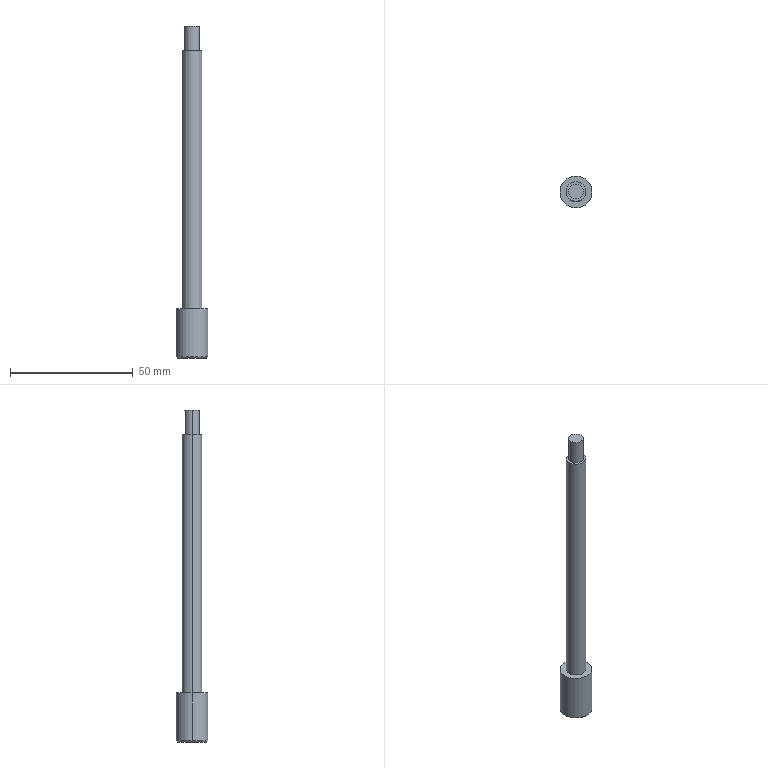Part | SolidWorks | features ICE 2, Chamfer 1, Extrusion 1, HoleWzd 1 | 1 solid | 20 faces | box 13 x 13 x 135 mm | volume 8178 mm3 | cylinder 10 | cone 6 | plane 4 | commonest cylinder face diameters 2 x4 6 x2 8 x2 13 x2
STEP:
#1=CARTESIAN_POINT('',(3.,0.,135.));
#2=VERTEX_POINT('',#1);
#3=CARTESIAN_POINT('',(-3.,0.,135.));
#4=VERTEX_POINT('',#3);
#5=CARTESIAN_POINT('',(0.,0.,135.));
#6=DIRECTION('',(0.,0.,1.));
#7=DIRECTION('',(1.,0.,0.));
#8=AXIS2_PLACEMENT_3D('',#5,#6,#7);
#9=CIRCLE('',#8,3.);
#10=EDGE_CURVE('',#2,#4,#9,.T.);
#11=ORIENTED_EDGE('',*,*,#10,.F.);
#12=CARTESIAN_POINT('',(3.,0.,125.));
#13=VERTEX_POINT('',#12);
#14=CARTESIAN_POINT('',(3.,0.,135.));
#15=DIRECTION('',(0.,0.,-1.));
#16=VECTOR('',#15,1000.);
#17=LINE('',#14,#16);
#18=EDGE_CURVE('',#2,#13,#17,.T.);
#19=ORIENTED_EDGE('',*,*,#18,.T.);
#20=CARTESIAN_POINT('',(-3.,0.,125.));
#21=VERTEX_POINT('',#20);
#22=CARTESIAN_POINT('',(0.,0.,125.));
#23=DIRECTION('',(0.,0.,1.));
#24=DIRECTION('',(1.,0.,0.));
#25=AXIS2_PLACEMENT_3D('',#22,#23,#24);
#26=CIRCLE('',#25,3.);
#27=EDGE_CURVE('',#13,#21,#26,.T.);
#28=ORIENTED_EDGE('',*,*,#27,.T.);
#29=CARTESIAN_POINT('',(-3.,0.,135.));
#30=DIRECTION('',(0.,0.,-1.));
#31=VECTOR('',#30,1000.);
#32=LINE('',#29,#31);
#33=EDGE_CURVE('',#4,#21,#32,.T.);
#34=ORIENTED_EDGE('',*,*,#33,.F.);
#35=EDGE_LOOP('',(#11,#19,#28,#34));
#36=FACE_OUTER_BOUND('',#35,.T.);
#37=CARTESIAN_POINT('',(0.,0.,135.));
#38=DIRECTION('',(0.,0.,-1.));
#39=DIRECTION('',(-1.,0.,0.));
#40=AXIS2_PLACEMENT_3D('',#37,#38,#39);
#41=CYLINDRICAL_SURFACE('',#40,3.);
#42=ADVANCED_FACE('',(#36),#41,.T.);
#43=CARTESIAN_POINT('',(4.,0.,125.));
#44=VERTEX_POINT('',#43);
#45=CARTESIAN_POINT('',(-4.,0.,125.));
#46=VERTEX_POINT('',#45);
#47=CARTESIAN_POINT('',(0.,0.,125.));
#48=DIRECTION('',(0.,0.,1.));
#49=DIRECTION('',(1.,0.,0.));
#50=AXIS2_PLACEMENT_3D('',#47,#48,#49);
#51=CIRCLE('',#50,4.);
#52=EDGE_CURVE('',#44,#46,#51,.T.);
#53=ORIENTED_EDGE('',*,*,#52,.F.);
#54=CARTESIAN_POINT('',(4.,0.,20.));
#55=VERTEX_POINT('',#54);
#56=CARTESIAN_POINT('',(4.,0.,125.));
#57=DIRECTION('',(0.,0.,-1.));
#58=VECTOR('',#57,1000.);
#59=LINE('',#56,#58);
#60=EDGE_CURVE('',#44,#55,#59,.T.);
#61=ORIENTED_EDGE('',*,*,#60,.T.);
#62=CARTESIAN_POINT('',(-4.,0.,20.));
#63=VERTEX_POINT('',#62);
#64=CARTESIAN_POINT('',(0.,0.,20.));
#65=DIRECTION('',(0.,0.,1.));
#66=DIRECTION('',(1.,0.,0.));
#67=AXIS2_PLACEMENT_3D('',#64,#65,#66);
#68=CIRCLE('',#67,4.);
#69=EDGE_CURVE('',#55,#63,#68,.T.);
#70=ORIENTED_EDGE('',*,*,#69,.T.);
#71=CARTESIAN_POINT('',(-4.,0.,125.));
#72=DIRECTION('',(0.,0.,-1.));
#73=VECTOR('',#72,1000.);
#74=LINE('',#71,#73);
#75=EDGE_CURVE('',#46,#63,#74,.T.);
#76=ORIENTED_EDGE('',*,*,#75,.F.);
#77=EDGE_LOOP('',(#53,#61,#70,#76));
#78=FACE_OUTER_BOUND('',#77,.T.);
#79=CARTESIAN_POINT('',(0.,0.,125.));
#80=DIRECTION('',(0.,0.,-1.));
#81=DIRECTION('',(-1.,0.,0.));
#82=AXIS2_PLACEMENT_3D('',#79,#80,#81);
#83=CYLINDRICAL_SURFACE('',#82,4.);
#84=ADVANCED_FACE('',(#78),#83,.T.);
#85=CARTESIAN_POINT('',(4.5,0.,5.));
#86=VERTEX_POINT('',#85);
#87=CARTESIAN_POINT('',(2.5,0.,5.));
#88=VERTEX_POINT('',#87);
#89=CARTESIAN_POINT('',(3.5,0.,5.));
#90=DIRECTION('',(0.,0.,-1.));
#91=DIRECTION('',(-1.,0.,0.));
#92=AXIS2_PLACEMENT_3D('',#89,#90,#91);
#93=CIRCLE('',#92,1.);
#94=EDGE_CURVE('',#86,#88,#93,.T.);
#95=ORIENTED_EDGE('',*,*,#94,.F.);
#96=CARTESIAN_POINT('',(4.5,0.,0.));
#97=VERTEX_POINT('',#96);
#98=CARTESIAN_POINT('',(4.5,0.,0.));
#99=DIRECTION('',(0.,0.,-1.));
#100=VECTOR('',#99,1000.);
#101=LINE('',#98,#100);
#102=EDGE_CURVE('',#86,#97,#101,.T.);
#103=ORIENTED_EDGE('',*,*,#102,.T.);
#104=CARTESIAN_POINT('',(2.5,0.,0.));
#105=VERTEX_POINT('',#104);
#106=CARTESIAN_POINT('',(3.5,0.,0.));
#107=DIRECTION('',(0.,0.,-1.));
#108=DIRECTION('',(-1.,0.,0.));
#109=AXIS2_PLACEMENT_3D('',#106,#107,#108);
#110=CIRCLE('',#109,1.);
#111=EDGE_CURVE('',#97,#105,#110,.T.);
#112=ORIENTED_EDGE('',*,*,#111,.T.);
#113=CARTESIAN_POINT('',(2.5,0.,0.));
#114=DIRECTION('',(0.,0.,-1.));
#115=VECTOR('',#114,1000.);
#116=LINE('',#113,#115);
#117=EDGE_CURVE('',#88,#105,#116,.T.);
#118=ORIENTED_EDGE('',*,*,#117,.F.);
#119=EDGE_LOOP('',(#95,#103,#112,#118));
#120=FACE_OUTER_BOUND('',#119,.T.);
#121=CARTESIAN_POINT('',(3.5,0.,0.));
#122=DIRECTION('',(0.,0.,-1.));
#123=DIRECTION('',(-1.,0.,0.));
#124=AXIS2_PLACEMENT_3D('',#121,#122,#123);
#125=CYLINDRICAL_SURFACE('',#124,1.);
#126=ADVANCED_FACE('',(#120),#125,.F.);
#127=CARTESIAN_POINT('',(3.5,0.,5.601));
#128=VERTEX_POINT('',#127);
#129=CARTESIAN_POINT('',(2.5,0.,5.));
#130=DIRECTION('',(-0.8572,0.,-0.515));
#131=VECTOR('',#130,1000.);
#132=LINE('',#129,#131);
#133=EDGE_CURVE('',#128,#88,#132,.T.);
#134=ORIENTED_EDGE('',*,*,#133,.F.);
#135=CARTESIAN_POINT('',(4.5,0.,5.));
#136=DIRECTION('',(0.8572,0.,-0.515));
#137=VECTOR('',#136,1000.);
#138=LINE('',#135,#137);
#139=EDGE_CURVE('',#128,#86,#138,.T.);
#140=ORIENTED_EDGE('',*,*,#139,.T.);
#141=ORIENTED_EDGE('',*,*,#94,.T.);
#142=EDGE_LOOP('',(#134,#140,#141));
#143=FACE_OUTER_BOUND('',#142,.T.);
#144=CARTESIAN_POINT('',(3.5,0.,5.));
#145=DIRECTION('',(0.,0.,-1.));
#146=DIRECTION('',(-1.,0.,0.));
#147=AXIS2_PLACEMENT_3D('',#144,#145,#146);
#148=CONICAL_SURFACE('',#147,1.,1.03);
#149=ADVANCED_FACE('',(#143),#148,.F.);
#150=CARTESIAN_POINT('',(-2.5,0.,5.));
#151=VERTEX_POINT('',#150);
#152=CARTESIAN_POINT('',(-4.5,0.,5.));
#153=VERTEX_POINT('',#152);
#154=CARTESIAN_POINT('',(-3.5,0.,5.));
#155=DIRECTION('',(0.,0.,-1.));
#156=DIRECTION('',(-1.,0.,0.));
#157=AXIS2_PLACEMENT_3D('',#154,#155,#156);
#158=CIRCLE('',#157,1.);
#159=EDGE_CURVE('',#151,#153,#158,.T.);
#160=ORIENTED_EDGE('',*,*,#159,.F.);
#161=CARTESIAN_POINT('',(-2.5,0.,0.));
#162=VERTEX_POINT('',#161);
#163=CARTESIAN_POINT('',(-2.5,0.,0.));
#164=DIRECTION('',(0.,0.,-1.));
#165=VECTOR('',#164,1000.);
#166=LINE('',#163,#165);
#167=EDGE_CURVE('',#151,#162,#166,.T.);
#168=ORIENTED_EDGE('',*,*,#167,.T.);
#169=CARTESIAN_POINT('',(-4.5,0.,0.));
#170=VERTEX_POINT('',#169);
#171=CARTESIAN_POINT('',(-3.5,0.,0.));
#172=DIRECTION('',(0.,0.,-1.));
#173=DIRECTION('',(-1.,0.,0.));
#174=AXIS2_PLACEMENT_3D('',#171,#172,#173);
#175=CIRCLE('',#174,1.);
#176=EDGE_CURVE('',#162,#170,#175,.T.);
#177=ORIENTED_EDGE('',*,*,#176,.T.);
#178=CARTESIAN_POINT('',(-4.5,0.,0.));
#179=DIRECTION('',(0.,0.,-1.));
#180=VECTOR('',#179,1000.);
#181=LINE('',#178,#180);
#182=EDGE_CURVE('',#153,#170,#181,.T.);
#183=ORIENTED_EDGE('',*,*,#182,.F.);
#184=EDGE_LOOP('',(#160,#168,#177,#183));
#185=FACE_OUTER_BOUND('',#184,.T.);
#186=CARTESIAN_POINT('',(-3.5,0.,0.));
#187=DIRECTION('',(0.,0.,-1.));
#188=DIRECTION('',(-1.,0.,0.));
#189=AXIS2_PLACEMENT_3D('',#186,#187,#188);
#190=CYLINDRICAL_SURFACE('',#189,1.);
#191=ADVANCED_FACE('',(#185),#190,.F.);
#192=CARTESIAN_POINT('',(-3.5,0.,5.601));
#193=VERTEX_POINT('',#192);
#194=CARTESIAN_POINT('',(-4.5,0.,5.));
#195=DIRECTION('',(-0.8572,0.,-0.515));
#196=VECTOR('',#195,1000.);
#197=LINE('',#194,#196);
#198=EDGE_CURVE('',#193,#153,#197,.T.);
#199=ORIENTED_EDGE('',*,*,#198,.F.);
#200=CARTESIAN_POINT('',(-2.5,0.,5.));
#201=DIRECTION('',(0.8572,0.,-0.515));
#202=VECTOR('',#201,1000.);
#203=LINE('',#200,#202);
#204=EDGE_CURVE('',#193,#151,#203,.T.);
#205=ORIENTED_EDGE('',*,*,#204,.T.);
#206=ORIENTED_EDGE('',*,*,#159,.T.);
#207=EDGE_LOOP('',(#199,#205,#206));
#208=FACE_OUTER_BOUND('',#207,.T.);
#209=CARTESIAN_POINT('',(-3.5,0.,5.));
#210=DIRECTION('',(0.,0.,-1.));
#211=DIRECTION('',(-1.,0.,0.));
#212=AXIS2_PLACEMENT_3D('',#209,#210,#211);
#213=CONICAL_SURFACE('',#212,1.,1.03);
#214=ADVANCED_FACE('',(#208),#213,.F.);
#215=CARTESIAN_POINT('',(-6.,0.,0.));
#216=VERTEX_POINT('',#215);
#217=CARTESIAN_POINT('',(6.,0.,0.));
#218=VERTEX_POINT('',#217);
#219=CARTESIAN_POINT('',(0.,0.,0.));
#220=DIRECTION('',(0.,0.,-1.));
#221=DIRECTION('',(1.,0.,0.));
#222=AXIS2_PLACEMENT_3D('',#219,#220,#221);
#223=CIRCLE('',#222,6.);
#224=EDGE_CURVE('',#216,#218,#223,.T.);
#225=ORIENTED_EDGE('',*,*,#224,.F.);
#226=CARTESIAN_POINT('',(-6.5,0.,0.5));
#227=VERTEX_POINT('',#226);
#228=CARTESIAN_POINT('',(-6.5,0.,0.5));
#229=DIRECTION('',(-0.7071,0.,0.7071));
#230=VECTOR('',#229,1000.);
#231=LINE('',#228,#230);
#232=EDGE_CURVE('',#216,#227,#231,.T.);
#233=ORIENTED_EDGE('',*,*,#232,.T.);
#234=CARTESIAN_POINT('',(6.5,0.,0.5));
#235=VERTEX_POINT('',#234);
#236=CARTESIAN_POINT('',(0.,0.,0.5));
#237=DIRECTION('',(0.,0.,1.));
#238=DIRECTION('',(1.,0.,0.));
#239=AXIS2_PLACEMENT_3D('',#236,#237,#238);
#240=CIRCLE('',#239,6.5);
#241=EDGE_CURVE('',#235,#227,#240,.T.);
#242=ORIENTED_EDGE('',*,*,#241,.F.);
#243=CARTESIAN_POINT('',(6.5,0.,0.5));
#244=DIRECTION('',(0.7071,0.,0.7071));
#245=VECTOR('',#244,1000.);
#246=LINE('',#243,#245);
#247=EDGE_CURVE('',#218,#235,#246,.T.);
#248=ORIENTED_EDGE('',*,*,#247,.F.);
#249=EDGE_LOOP('',(#225,#233,#242,#248));
#250=FACE_OUTER_BOUND('',#249,.T.);
#251=CARTESIAN_POINT('',(0.,0.,0.5));
#252=DIRECTION('',(0.,0.,1.));
#253=DIRECTION('',(1.,0.,0.));
#254=AXIS2_PLACEMENT_3D('',#251,#252,#253);
#255=CONICAL_SURFACE('',#254,6.5,0.7854);
#256=ADVANCED_FACE('',(#250),#255,.T.);
#257=CARTESIAN_POINT('',(6.5,0.,20.));
#258=VERTEX_POINT('',#257);
#259=CARTESIAN_POINT('',(-6.5,0.,20.));
#260=VERTEX_POINT('',#259);
#261=CARTESIAN_POINT('',(0.,0.,20.));
#262=DIRECTION('',(0.,0.,1.));
#263=DIRECTION('',(1.,0.,0.));
#264=AXIS2_PLACEMENT_3D('',#261,#262,#263);
#265=CIRCLE('',#264,6.5);
#266=EDGE_CURVE('',#258,#260,#265,.T.);
#267=ORIENTED_EDGE('',*,*,#266,.F.);
#268=CARTESIAN_POINT('',(6.5,0.,20.));
#269=DIRECTION('',(0.,0.,-1.));
#270=VECTOR('',#269,1000.);
#271=LINE('',#268,#270);
#272=EDGE_CURVE('',#258,#235,#271,.T.);
#273=ORIENTED_EDGE('',*,*,#272,.T.);
#274=ORIENTED_EDGE('',*,*,#241,.T.);
#275=CARTESIAN_POINT('',(-6.5,0.,20.));
#276=DIRECTION('',(0.,0.,-1.));
#277=VECTOR('',#276,1000.);
#278=LINE('',#275,#277);
#279=EDGE_CURVE('',#260,#227,#278,.T.);
#280=ORIENTED_EDGE('',*,*,#279,.F.);
#281=EDGE_LOOP('',(#267,#273,#274,#280));
#282=FACE_OUTER_BOUND('',#281,.T.);
#283=CARTESIAN_POINT('',(0.,0.,20.));
#284=DIRECTION('',(0.,0.,-1.));
#285=DIRECTION('',(-1.,0.,0.));
#286=AXIS2_PLACEMENT_3D('',#283,#284,#285);
#287=CYLINDRICAL_SURFACE('',#286,6.5);
#288=ADVANCED_FACE('',(#282),#287,.T.);
#289=ORIENTED_EDGE('',*,*,#272,.F.);
#290=CARTESIAN_POINT('',(0.,0.,20.));
#291=DIRECTION('',(0.,0.,1.));
#292=DIRECTION('',(1.,0.,0.));
#293=AXIS2_PLACEMENT_3D('',#290,#291,#292);
#294=CIRCLE('',#293,6.5);
#295=EDGE_CURVE('',#260,#258,#294,.T.);
#296=ORIENTED_EDGE('',*,*,#295,.F.);
#297=ORIENTED_EDGE('',*,*,#279,.T.);
#298=CARTESIAN_POINT('',(0.,0.,0.5));
#299=DIRECTION('',(0.,0.,1.));
#300=DIRECTION('',(1.,0.,0.));
#301=AXIS2_PLACEMENT_3D('',#298,#299,#300);
#302=CIRCLE('',#301,6.5);
#303=EDGE_CURVE('',#227,#235,#302,.T.);
#304=ORIENTED_EDGE('',*,*,#303,.T.);
#305=EDGE_LOOP('',(#289,#296,#297,#304));
#306=FACE_OUTER_BOUND('',#305,.T.);
#307=CARTESIAN_POINT('',(0.,0.,20.));
#308=DIRECTION('',(0.,0.,-1.));
#309=DIRECTION('',(-1.,0.,0.));
#310=AXIS2_PLACEMENT_3D('',#307,#308,#309);
#311=CYLINDRICAL_SURFACE('',#310,6.5);
#312=ADVANCED_FACE('',(#306),#311,.T.);
#313=CARTESIAN_POINT('',(0.,0.,20.));
#314=DIRECTION('',(0.,0.,1.));
#315=DIRECTION('',(1.,0.,0.));
#316=AXIS2_PLACEMENT_3D('',#313,#314,#315);
#317=CIRCLE('',#316,4.);
#318=EDGE_CURVE('',#63,#55,#317,.T.);
#319=ORIENTED_EDGE('',*,*,#318,.F.);
#320=ORIENTED_EDGE('',*,*,#69,.F.);
#321=EDGE_LOOP('',(#319,#320));
#322=FACE_BOUND('',#321,.T.);
#323=ORIENTED_EDGE('',*,*,#295,.T.);
#324=ORIENTED_EDGE('',*,*,#266,.T.);
#325=EDGE_LOOP('',(#323,#324));
#326=FACE_OUTER_BOUND('',#325,.T.);
#327=CARTESIAN_POINT('',(0.,0.,20.));
#328=DIRECTION('',(0.,0.,1.));
#329=DIRECTION('',(1.,0.,0.));
#330=AXIS2_PLACEMENT_3D('',#327,#328,#329);
#331=PLANE('',#330);
#332=ADVANCED_FACE('',(#322,#326),#331,.T.);
#333=CARTESIAN_POINT('',(3.5,0.,0.));
#334=DIRECTION('',(0.,0.,-1.));
#335=DIRECTION('',(-1.,0.,0.));
#336=AXIS2_PLACEMENT_3D('',#333,#334,#335);
#337=CIRCLE('',#336,1.);
#338=EDGE_CURVE('',#105,#97,#337,.T.);
#339=ORIENTED_EDGE('',*,*,#338,.F.);
#340=ORIENTED_EDGE('',*,*,#111,.F.);
#341=EDGE_LOOP('',(#339,#340));
#342=FACE_BOUND('',#341,.T.);
#343=CARTESIAN_POINT('',(-3.5,0.,0.));
#344=DIRECTION('',(0.,0.,-1.));
#345=DIRECTION('',(-1.,0.,0.));
#346=AXIS2_PLACEMENT_3D('',#343,#344,#345);
#347=CIRCLE('',#346,1.);
#348=EDGE_CURVE('',#170,#162,#347,.T.);
#349=ORIENTED_EDGE('',*,*,#348,.F.);
#350=ORIENTED_EDGE('',*,*,#176,.F.);
#351=EDGE_LOOP('',(#349,#350));
#352=FACE_BOUND('',#351,.T.);
#353=CARTESIAN_POINT('',(0.,0.,0.));
#354=DIRECTION('',(0.,0.,-1.));
#355=DIRECTION('',(1.,0.,0.));
#356=AXIS2_PLACEMENT_3D('',#353,#354,#355);
#357=CIRCLE('',#356,6.);
#358=EDGE_CURVE('',#218,#216,#357,.T.);
#359=ORIENTED_EDGE('',*,*,#358,.T.);
#360=ORIENTED_EDGE('',*,*,#224,.T.);
#361=EDGE_LOOP('',(#359,#360));
#362=FACE_OUTER_BOUND('',#361,.T.);
#363=CARTESIAN_POINT('',(0.,0.,0.));
#364=DIRECTION('',(0.,0.,1.));
#365=DIRECTION('',(1.,0.,0.));
#366=AXIS2_PLACEMENT_3D('',#363,#364,#365);
#367=PLANE('',#366);
#368=ADVANCED_FACE('',(#342,#352,#362),#367,.F.);
#369=ORIENTED_EDGE('',*,*,#232,.F.);
#370=ORIENTED_EDGE('',*,*,#358,.F.);
#371=ORIENTED_EDGE('',*,*,#247,.T.);
#372=ORIENTED_EDGE('',*,*,#303,.F.);
#373=EDGE_LOOP('',(#369,#370,#371,#372));
#374=FACE_OUTER_BOUND('',#373,.T.);
#375=CARTESIAN_POINT('',(0.,0.,0.5));
#376=DIRECTION('',(0.,0.,1.));
#377=DIRECTION('',(1.,0.,0.));
#378=AXIS2_PLACEMENT_3D('',#375,#376,#377);
#379=CONICAL_SURFACE('',#378,6.5,0.7854);
#380=ADVANCED_FACE('',(#374),#379,.T.);
#381=ORIENTED_EDGE('',*,*,#204,.F.);
#382=ORIENTED_EDGE('',*,*,#198,.T.);
#383=CARTESIAN_POINT('',(-3.5,0.,5.));
#384=DIRECTION('',(0.,0.,-1.));
#385=DIRECTION('',(-1.,0.,0.));
#386=AXIS2_PLACEMENT_3D('',#383,#384,#385);
#387=CIRCLE('',#386,1.);
#388=EDGE_CURVE('',#153,#151,#387,.T.);
#389=ORIENTED_EDGE('',*,*,#388,.T.);
#390=EDGE_LOOP('',(#381,#382,#389));
#391=FACE_OUTER_BOUND('',#390,.T.);
#392=CARTESIAN_POINT('',(-3.5,0.,5.));
#393=DIRECTION('',(0.,0.,-1.));
#394=DIRECTION('',(-1.,0.,0.));
#395=AXIS2_PLACEMENT_3D('',#392,#393,#394);
#396=CONICAL_SURFACE('',#395,1.,1.03);
#397=ADVANCED_FACE('',(#391),#396,.F.);
#398=ORIENTED_EDGE('',*,*,#167,.F.);
#399=ORIENTED_EDGE('',*,*,#388,.F.);
#400=ORIENTED_EDGE('',*,*,#182,.T.);
#401=ORIENTED_EDGE('',*,*,#348,.T.);
#402=EDGE_LOOP('',(#398,#399,#400,#401));
#403=FACE_OUTER_BOUND('',#402,.T.);
#404=CARTESIAN_POINT('',(-3.5,0.,0.));
#405=DIRECTION('',(0.,0.,-1.));
#406=DIRECTION('',(-1.,0.,0.));
#407=AXIS2_PLACEMENT_3D('',#404,#405,#406);
#408=CYLINDRICAL_SURFACE('',#407,1.);
#409=ADVANCED_FACE('',(#403),#408,.F.);
#410=ORIENTED_EDGE('',*,*,#139,.F.);
#411=ORIENTED_EDGE('',*,*,#133,.T.);
#412=CARTESIAN_POINT('',(3.5,0.,5.));
#413=DIRECTION('',(0.,0.,-1.));
#414=DIRECTION('',(-1.,0.,0.));
#415=AXIS2_PLACEMENT_3D('',#412,#413,#414);
#416=CIRCLE('',#415,1.);
#417=EDGE_CURVE('',#88,#86,#416,.T.);
#418=ORIENTED_EDGE('',*,*,#417,.T.);
#419=EDGE_LOOP('',(#410,#411,#418));
#420=FACE_OUTER_BOUND('',#419,.T.);
#421=CARTESIAN_POINT('',(3.5,0.,5.));
#422=DIRECTION('',(0.,0.,-1.));
#423=DIRECTION('',(-1.,0.,0.));
#424=AXIS2_PLACEMENT_3D('',#421,#422,#423);
#425=CONICAL_SURFACE('',#424,1.,1.03);
#426=ADVANCED_FACE('',(#420),#425,.F.);
#427=ORIENTED_EDGE('',*,*,#102,.F.);
#428=ORIENTED_EDGE('',*,*,#417,.F.);
#429=ORIENTED_EDGE('',*,*,#117,.T.);
#430=ORIENTED_EDGE('',*,*,#338,.T.);
#431=EDGE_LOOP('',(#427,#428,#429,#430));
#432=FACE_OUTER_BOUND('',#431,.T.);
#433=CARTESIAN_POINT('',(3.5,0.,0.));
#434=DIRECTION('',(0.,0.,-1.));
#435=DIRECTION('',(-1.,0.,0.));
#436=AXIS2_PLACEMENT_3D('',#433,#434,#435);
#437=CYLINDRICAL_SURFACE('',#436,1.);
#438=ADVANCED_FACE('',(#432),#437,.F.);
#439=ORIENTED_EDGE('',*,*,#60,.F.);
#440=CARTESIAN_POINT('',(0.,0.,125.));
#441=DIRECTION('',(0.,0.,1.));
#442=DIRECTION('',(1.,0.,0.));
#443=AXIS2_PLACEMENT_3D('',#440,#441,#442);
#444=CIRCLE('',#443,4.);
#445=EDGE_CURVE('',#46,#44,#444,.T.);
#446=ORIENTED_EDGE('',*,*,#445,.F.);
#447=ORIENTED_EDGE('',*,*,#75,.T.);
#448=ORIENTED_EDGE('',*,*,#318,.T.);
#449=EDGE_LOOP('',(#439,#446,#447,#448));
#450=FACE_OUTER_BOUND('',#449,.T.);
#451=CARTESIAN_POINT('',(0.,0.,125.));
#452=DIRECTION('',(0.,0.,-1.));
#453=DIRECTION('',(-1.,0.,0.));
#454=AXIS2_PLACEMENT_3D('',#451,#452,#453);
#455=CYLINDRICAL_SURFACE('',#454,4.);
#456=ADVANCED_FACE('',(#450),#455,.T.);
#457=CARTESIAN_POINT('',(0.,0.,125.));
#458=DIRECTION('',(0.,0.,1.));
#459=DIRECTION('',(1.,0.,0.));
#460=AXIS2_PLACEMENT_3D('',#457,#458,#459);
#461=CIRCLE('',#460,3.);
#462=EDGE_CURVE('',#21,#13,#461,.T.);
#463=ORIENTED_EDGE('',*,*,#462,.F.);
#464=ORIENTED_EDGE('',*,*,#27,.F.);
#465=EDGE_LOOP('',(#463,#464));
#466=FACE_BOUND('',#465,.T.);
#467=ORIENTED_EDGE('',*,*,#445,.T.);
#468=ORIENTED_EDGE('',*,*,#52,.T.);
#469=EDGE_LOOP('',(#467,#468));
#470=FACE_OUTER_BOUND('',#469,.T.);
#471=CARTESIAN_POINT('',(0.,0.,125.));
#472=DIRECTION('',(0.,0.,1.));
#473=DIRECTION('',(1.,0.,0.));
#474=AXIS2_PLACEMENT_3D('',#471,#472,#473);
#475=PLANE('',#474);
#476=ADVANCED_FACE('',(#466,#470),#475,.T.);
#477=ORIENTED_EDGE('',*,*,#18,.F.);
#478=CARTESIAN_POINT('',(0.,0.,135.));
#479=DIRECTION('',(0.,0.,1.));
#480=DIRECTION('',(1.,0.,0.));
#481=AXIS2_PLACEMENT_3D('',#478,#479,#480);
#482=CIRCLE('',#481,3.);
#483=EDGE_CURVE('',#4,#2,#482,.T.);
#484=ORIENTED_EDGE('',*,*,#483,.F.);
#485=ORIENTED_EDGE('',*,*,#33,.T.);
#486=ORIENTED_EDGE('',*,*,#462,.T.);
#487=EDGE_LOOP('',(#477,#484,#485,#486));
#488=FACE_OUTER_BOUND('',#487,.T.);
#489=CARTESIAN_POINT('',(0.,0.,135.));
#490=DIRECTION('',(0.,0.,-1.));
#491=DIRECTION('',(-1.,0.,0.));
#492=AXIS2_PLACEMENT_3D('',#489,#490,#491);
#493=CYLINDRICAL_SURFACE('',#492,3.);
#494=ADVANCED_FACE('',(#488),#493,.T.);
#495=ORIENTED_EDGE('',*,*,#483,.T.);
#496=ORIENTED_EDGE('',*,*,#10,.T.);
#497=EDGE_LOOP('',(#495,#496));
#498=FACE_OUTER_BOUND('',#497,.T.);
#499=CARTESIAN_POINT('',(0.,0.,135.));
#500=DIRECTION('',(0.,0.,1.));
#501=DIRECTION('',(1.,0.,0.));
#502=AXIS2_PLACEMENT_3D('',#499,#500,#501);
#503=PLANE('',#502);
#504=ADVANCED_FACE('',(#498),#503,.T.);
#505=CLOSED_SHELL('',(#42,#84,#126,#149,#191,#214,#256,#288,#312,#332,#368,#380,#397,#409,#426,#438,#456,#476,#494,#504));
#506=MANIFOLD_SOLID_BREP('',#505);
#507=CARTESIAN_POINT('',(0.,0.,0.));
#508=DIRECTION('',(0.,0.,1.));
#509=DIRECTION('',(1.,0.,0.));
#510=AXIS2_PLACEMENT_3D('',#507,#508,#509);
#511=(LENGTH_UNIT()NAMED_UNIT(*)SI_UNIT(.MILLI.,.METRE.));
#512=UNCERTAINTY_MEASURE_WITH_UNIT(LENGTH_MEASURE(0.00001),#511,'','');
#513=(NAMED_UNIT(*)PLANE_ANGLE_UNIT()SI_UNIT($,.RADIAN.));
#514=(NAMED_UNIT(*)SI_UNIT($,.STERADIAN.)SOLID_ANGLE_UNIT());
#515=(GEOMETRIC_REPRESENTATION_CONTEXT(3)GLOBAL_UNCERTAINTY_ASSIGNED_CONTEXT((#512))GLOBAL_UNIT_ASSIGNED_CONTEXT((#511,#513,#514))REPRESENTATION_CONTEXT('',''));
#516=ADVANCED_BREP_SHAPE_REPRESENTATION('',(#506,#510),#515);